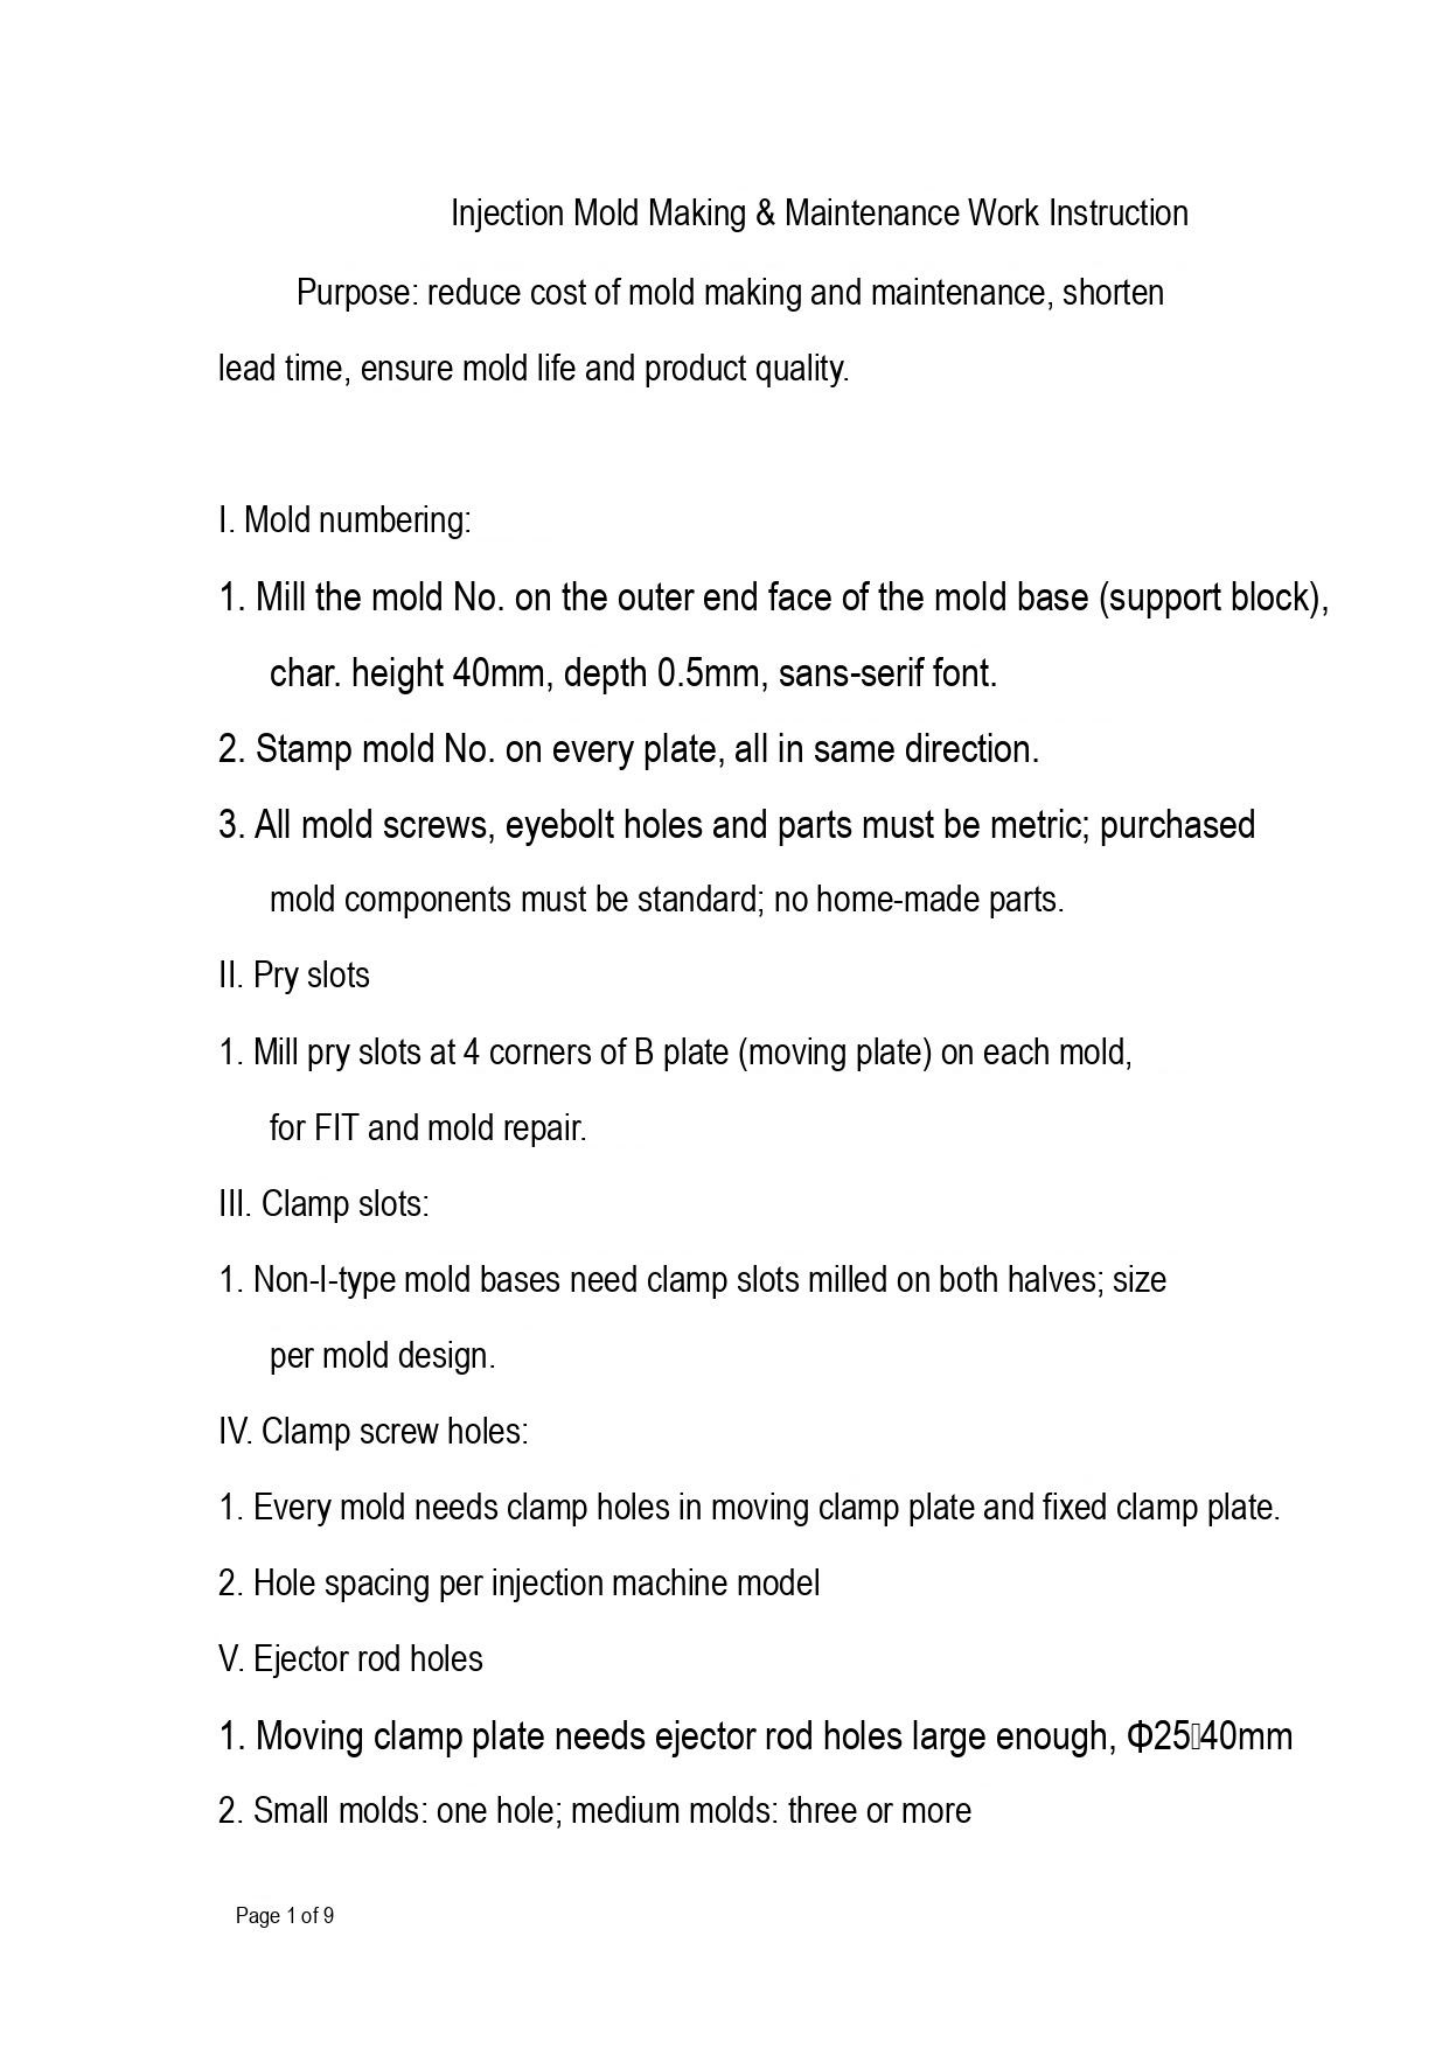Injection Mold Making & Maintenance Work Instruction

Purpose: reduce cost of mold making and maintenance, shorten lead time, ensure mold life and product quality.

I. Mold numbering:

1. Mill the mold No. on the outer end face of the mold base (support block), char. height 40mm, depth 0.5mm, sans-serif font.

2. Stamp mold No. on every plate, all in same direction.

3. All mold screws, eyebolt holes and parts must be metric; purchased mold components must be standard; no home-made parts.

II. Pry slots

1. Mill pry slots at 4 corners of B plate (moving plate) on each mold, for FIT and mold repair.

III. Clamp slots:

1. Non-I-type mold bases need clamp slots milled on both halves; size per mold design.

IV. Clamp screw holes:

1. Every mold needs clamp holes in moving clamp plate and fixed clamp plate.

2. Hole spacing per injection machine model

V. Ejector rod holes

1. Moving clamp plate needs ejector rod holes large enough, Φ25 40mm

2. Small molds: one hole; medium molds: three or more

Page 1 of 9
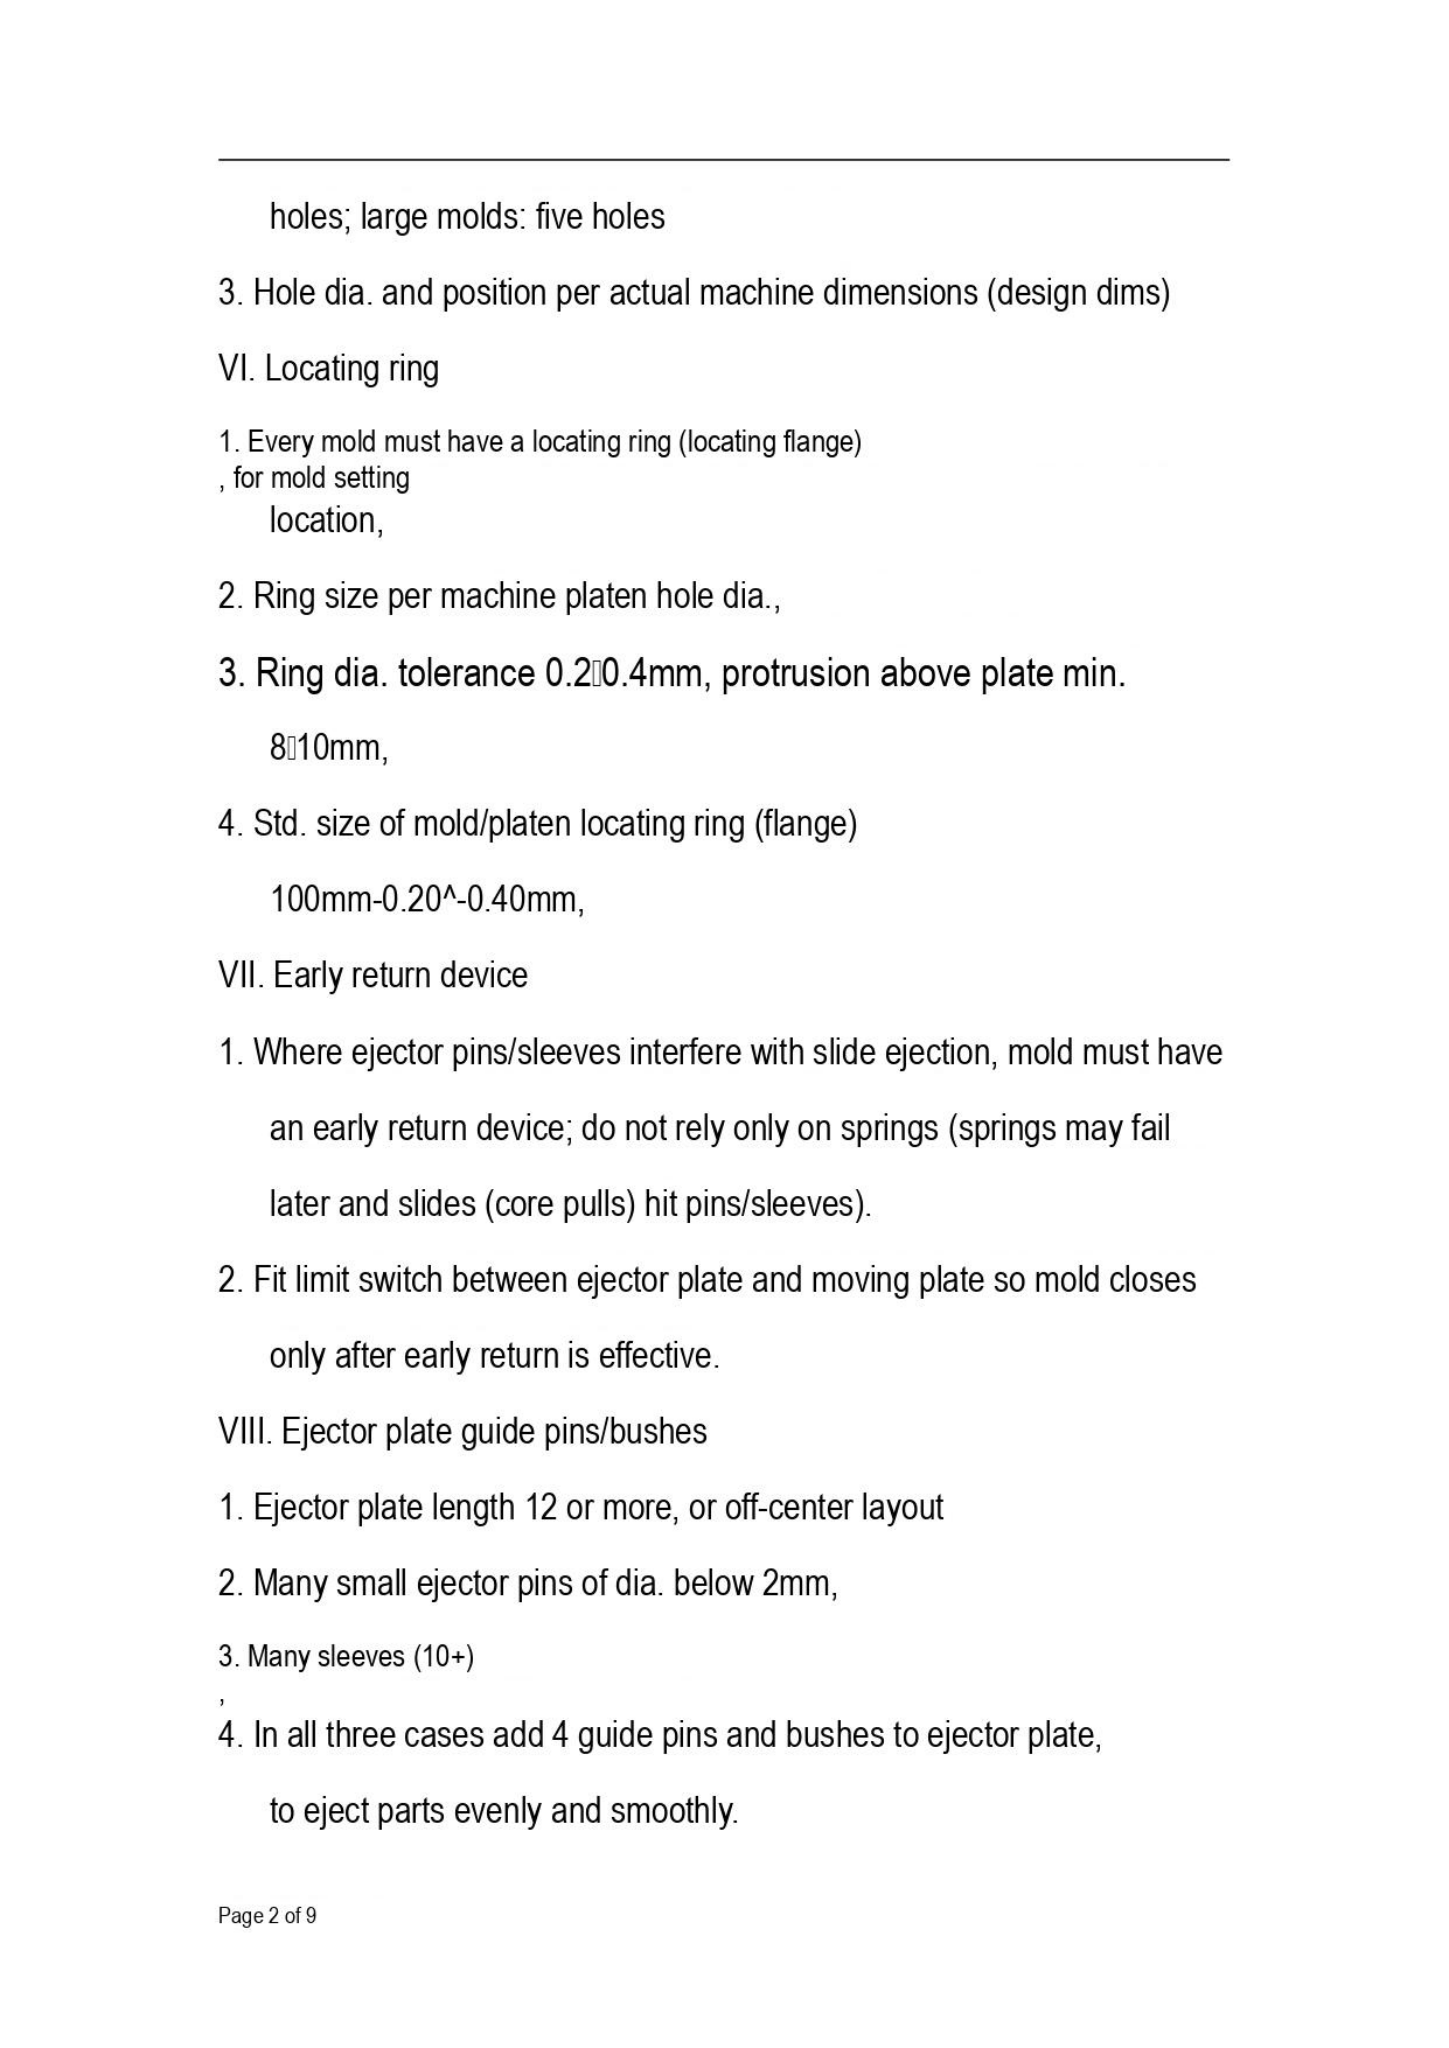holes; large molds: five holes

3. Hole dia. and position per actual machine dimensions (design dims)

VI. Locating ring

1. Every mold must have a locating ring (locating flange)
, for mold setting
location,

2. Ring size per machine platen hole dia.,

3. Ring dia. tolerance 0.2▯0.4mm, protrusion above plate min.
8▯10mm,

4. Std. size of mold/platen locating ring (flange)
100mm-0.20^-0.40mm,

VII. Early return device

1. Where ejector pins/sleeves interfere with slide ejection, mold must have an early return device; do not rely only on springs (springs may fail later and slides (core pulls) hit pins/sleeves).

2. Fit limit switch between ejector plate and moving plate so mold closes only after early return is effective.

VIII. Ejector plate guide pins/bushes

1. Ejector plate length 12 or more, or off-center layout

2. Many small ejector pins of dia. below 2mm,

3. Many sleeves (10+)
,

4. In all three cases add 4 guide pins and bushes to ejector plate, to eject parts evenly and smoothly.

Page 2 of 9
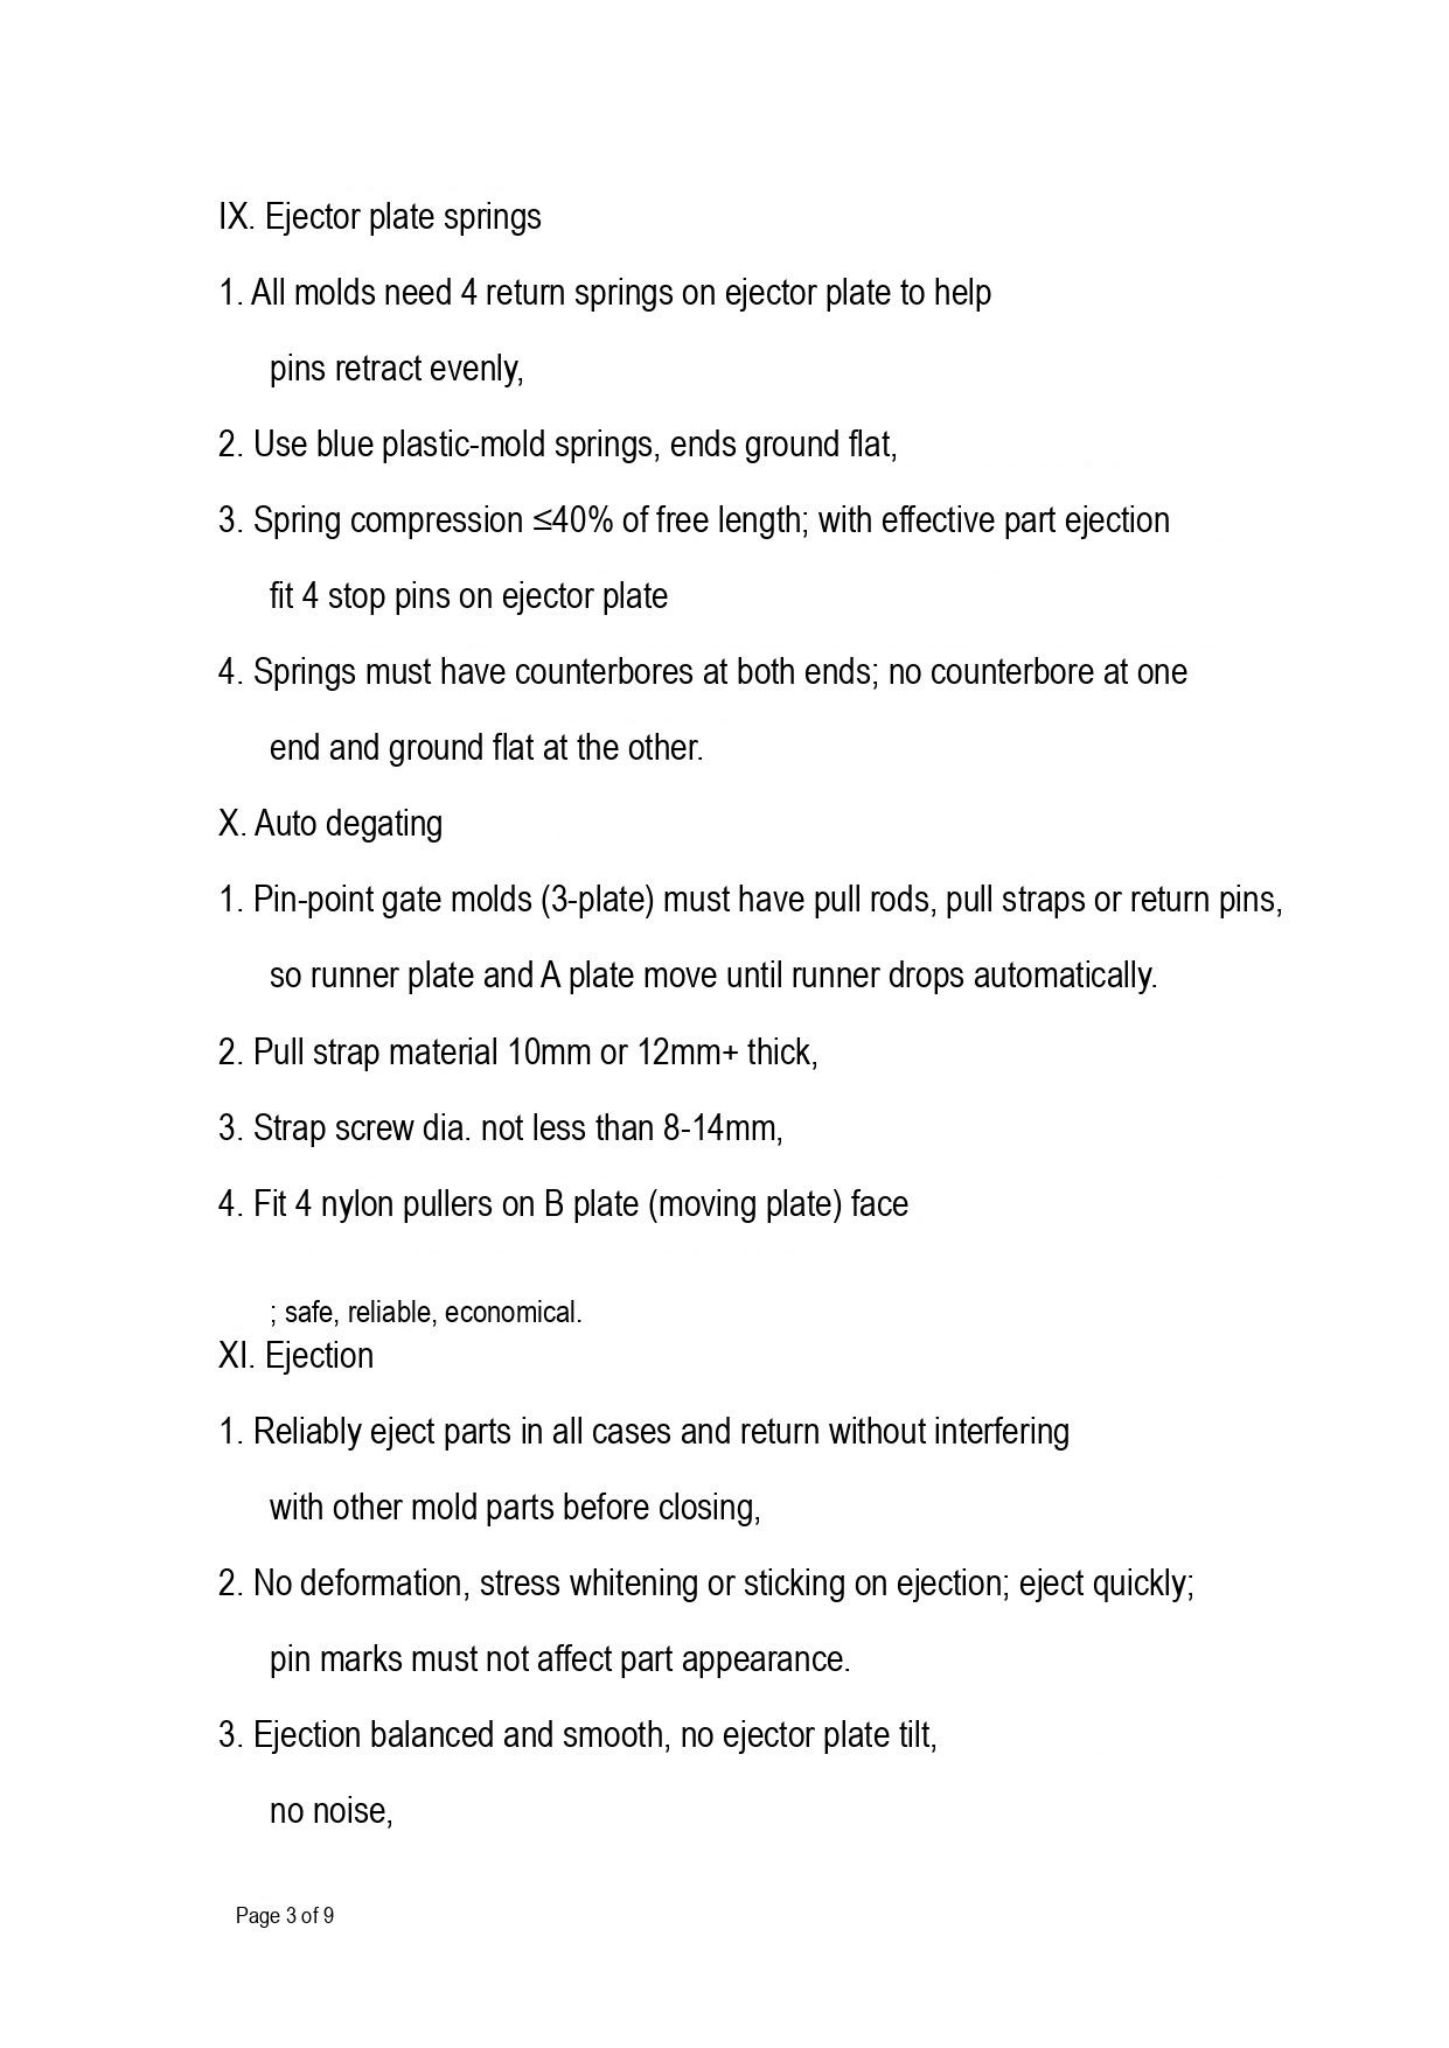IX. Ejector plate springs

1. All molds need 4 return springs on ejector plate to help
   pins retract evenly,

2. Use blue plastic-mold springs, ends ground flat,

3. Spring compression ≤40% of free length; with effective part ejection
   fit 4 stop pins on ejector plate

4. Springs must have counterbores at both ends; no counterbore at one
   end and ground flat at the other.

X. Auto degating

1. Pin-point gate molds (3-plate) must have pull rods, pull straps or return pins,
   so runner plate and A plate move until runner drops automatically.

2. Pull strap material 10mm or 12mm+ thick,

3. Strap screw dia. not less than 8-14mm,

4. Fit 4 nylon pullers on B plate (moving plate) face

   ; safe, reliable, economical.

XI. Ejection

1. Reliably eject parts in all cases and return without interfering
   with other mold parts before closing,

2. No deformation, stress whitening or sticking on ejection; eject quickly;
   pin marks must not affect part appearance.

3. Ejection balanced and smooth, no ejector plate tilt,
   no noise,

Page 3 of 9
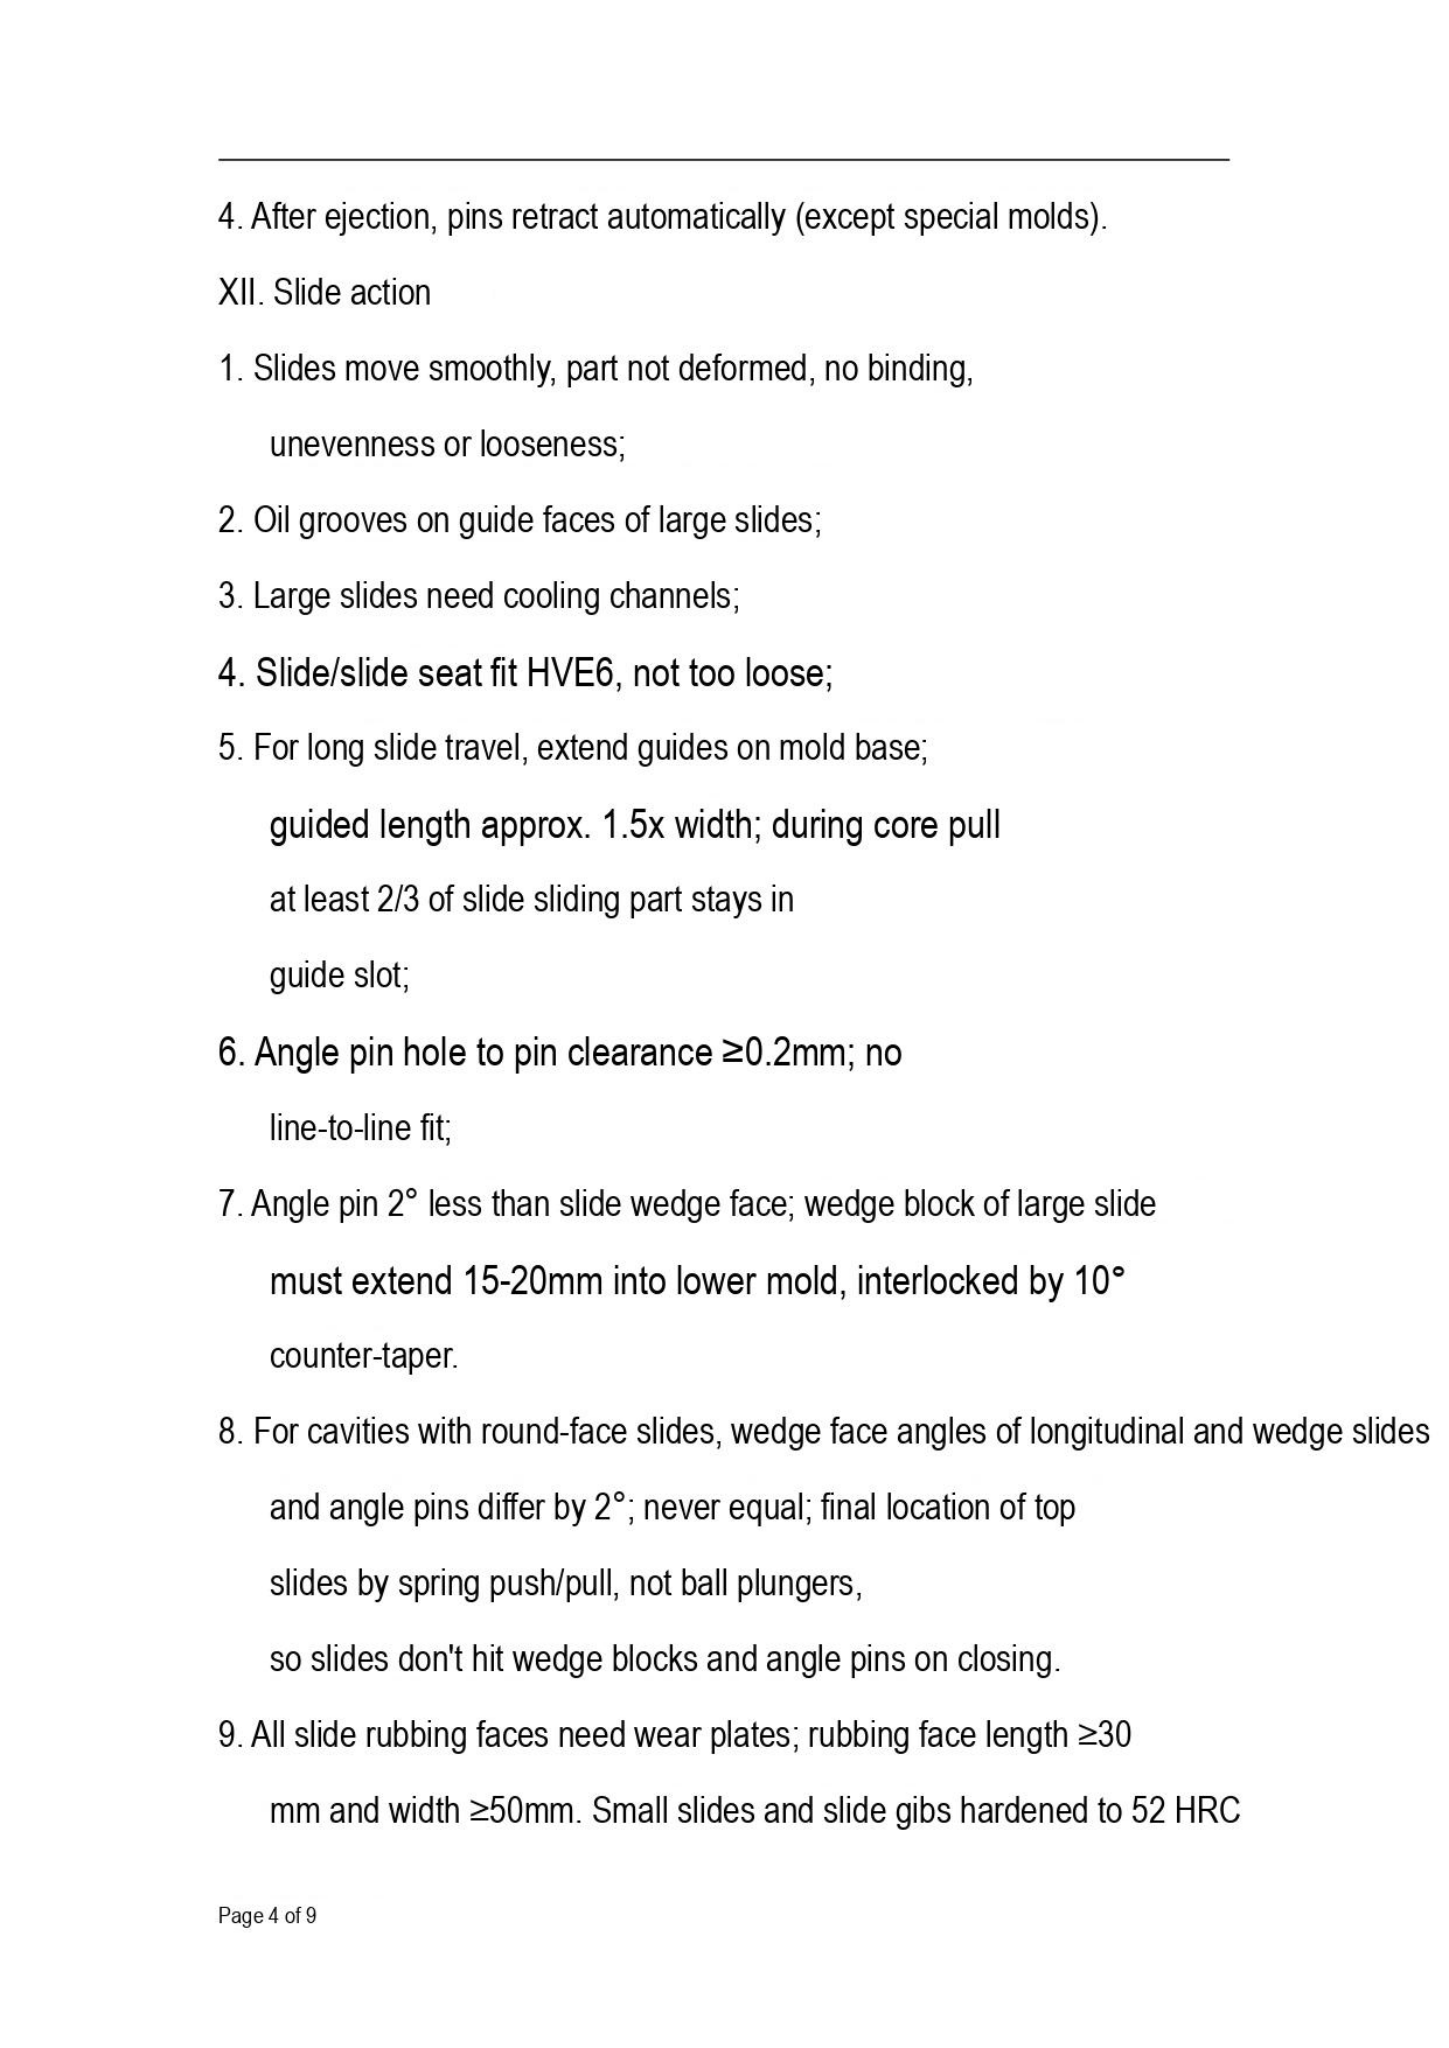4. After ejection, pins retract automatically (except special molds).

XII. Slide action

1. Slides move smoothly, part not deformed, no binding, unevenness or looseness;

2. Oil grooves on guide faces of large slides;

3. Large slides need cooling channels;

4. Slide/slide seat fit HVE6, not too loose;

5. For long slide travel, extend guides on mold base; guided length approx. 1.5x width; during core pull at least 2/3 of slide sliding part stays in guide slot;

6. Angle pin hole to pin clearance ≥0.2mm; no line-to-line fit;

7. Angle pin 2° less than slide wedge face; wedge block of large slide must extend 15-20mm into lower mold, interlocked by 10° counter-taper.

8. For cavities with round-face slides, wedge face angles of longitudinal and wedge slides and angle pins differ by 2°; never equal; final location of top slides by spring push/pull, not ball plungers, so slides don't hit wedge blocks and angle pins on closing.

9. All slide rubbing faces need wear plates; rubbing face length ≥30 mm and width ≥50mm. Small slides and slide gibs hardened to 52 HRC

Page 4 of 9
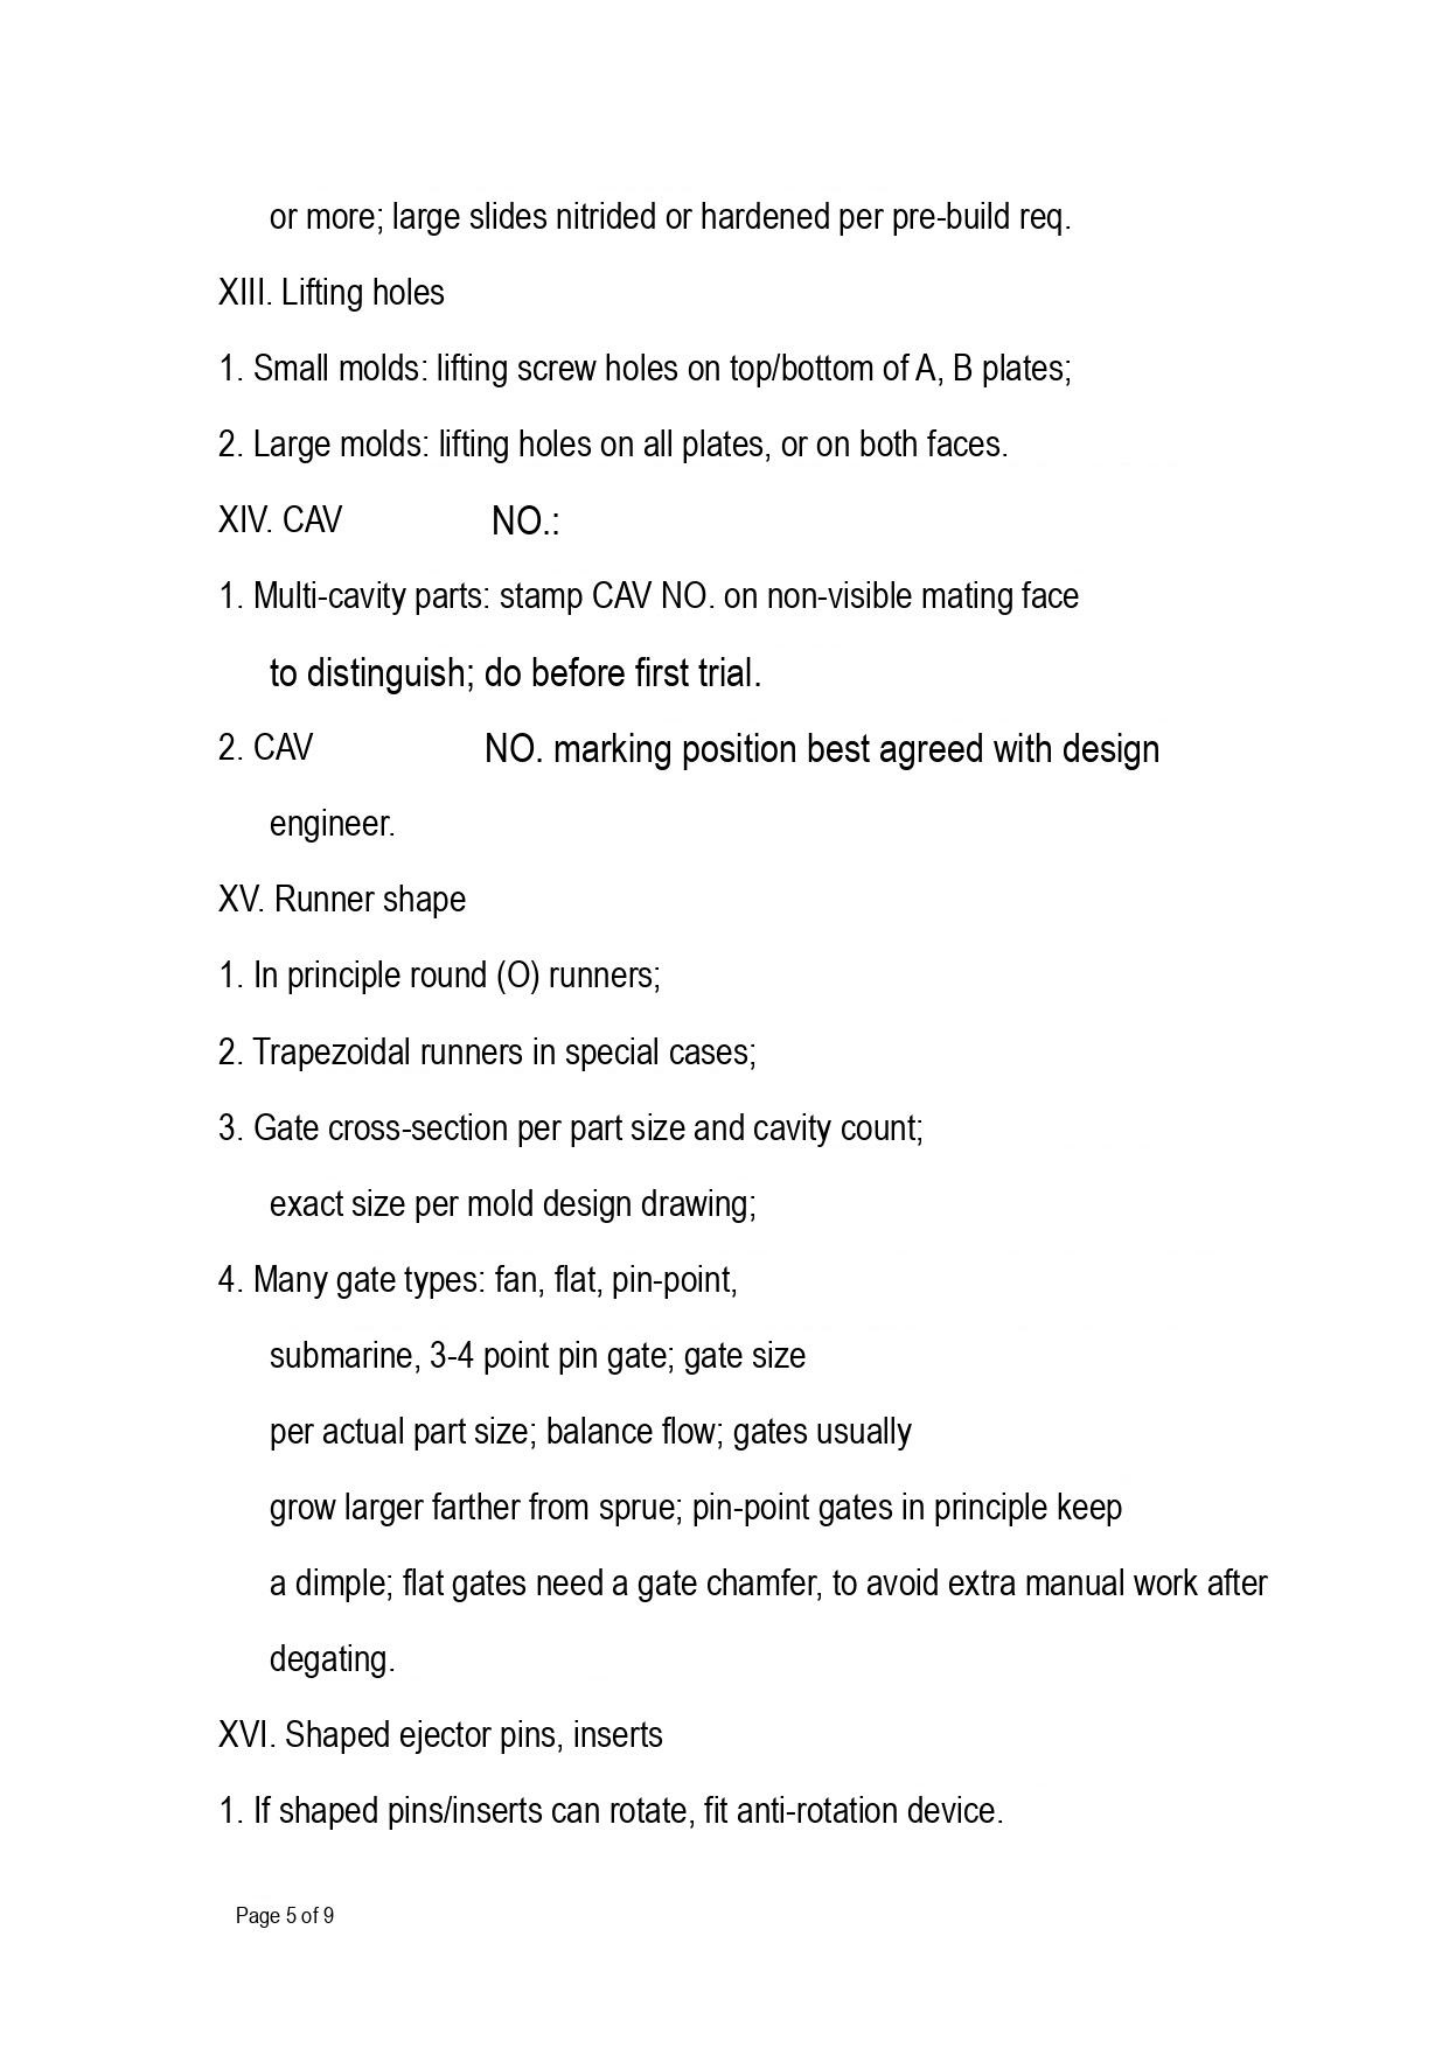or more; large slides nitrided or hardened per pre-build req.

XIII. Lifting holes

1. Small molds: lifting screw holes on top/bottom of A, B plates;

2. Large molds: lifting holes on all plates, or on both faces.

XIV. CAV NO.:

1. Multi-cavity parts: stamp CAV NO. on non-visible mating face to distinguish; do before first trial.

2. CAV NO. marking position best agreed with design engineer.

XV. Runner shape

1. In principle round (O) runners;

2. Trapezoidal runners in special cases;

3. Gate cross-section per part size and cavity count; exact size per mold design drawing;

4. Many gate types: fan, flat, pin-point, submarine, 3-4 point pin gate; gate size per actual part size; balance flow; gates usually grow larger farther from sprue; pin-point gates in principle keep a dimple; flat gates need a gate chamfer, to avoid extra manual work after degating.

XVI. Shaped ejector pins, inserts

1. If shaped pins/inserts can rotate, fit anti-rotation device.

Page 5 of 9
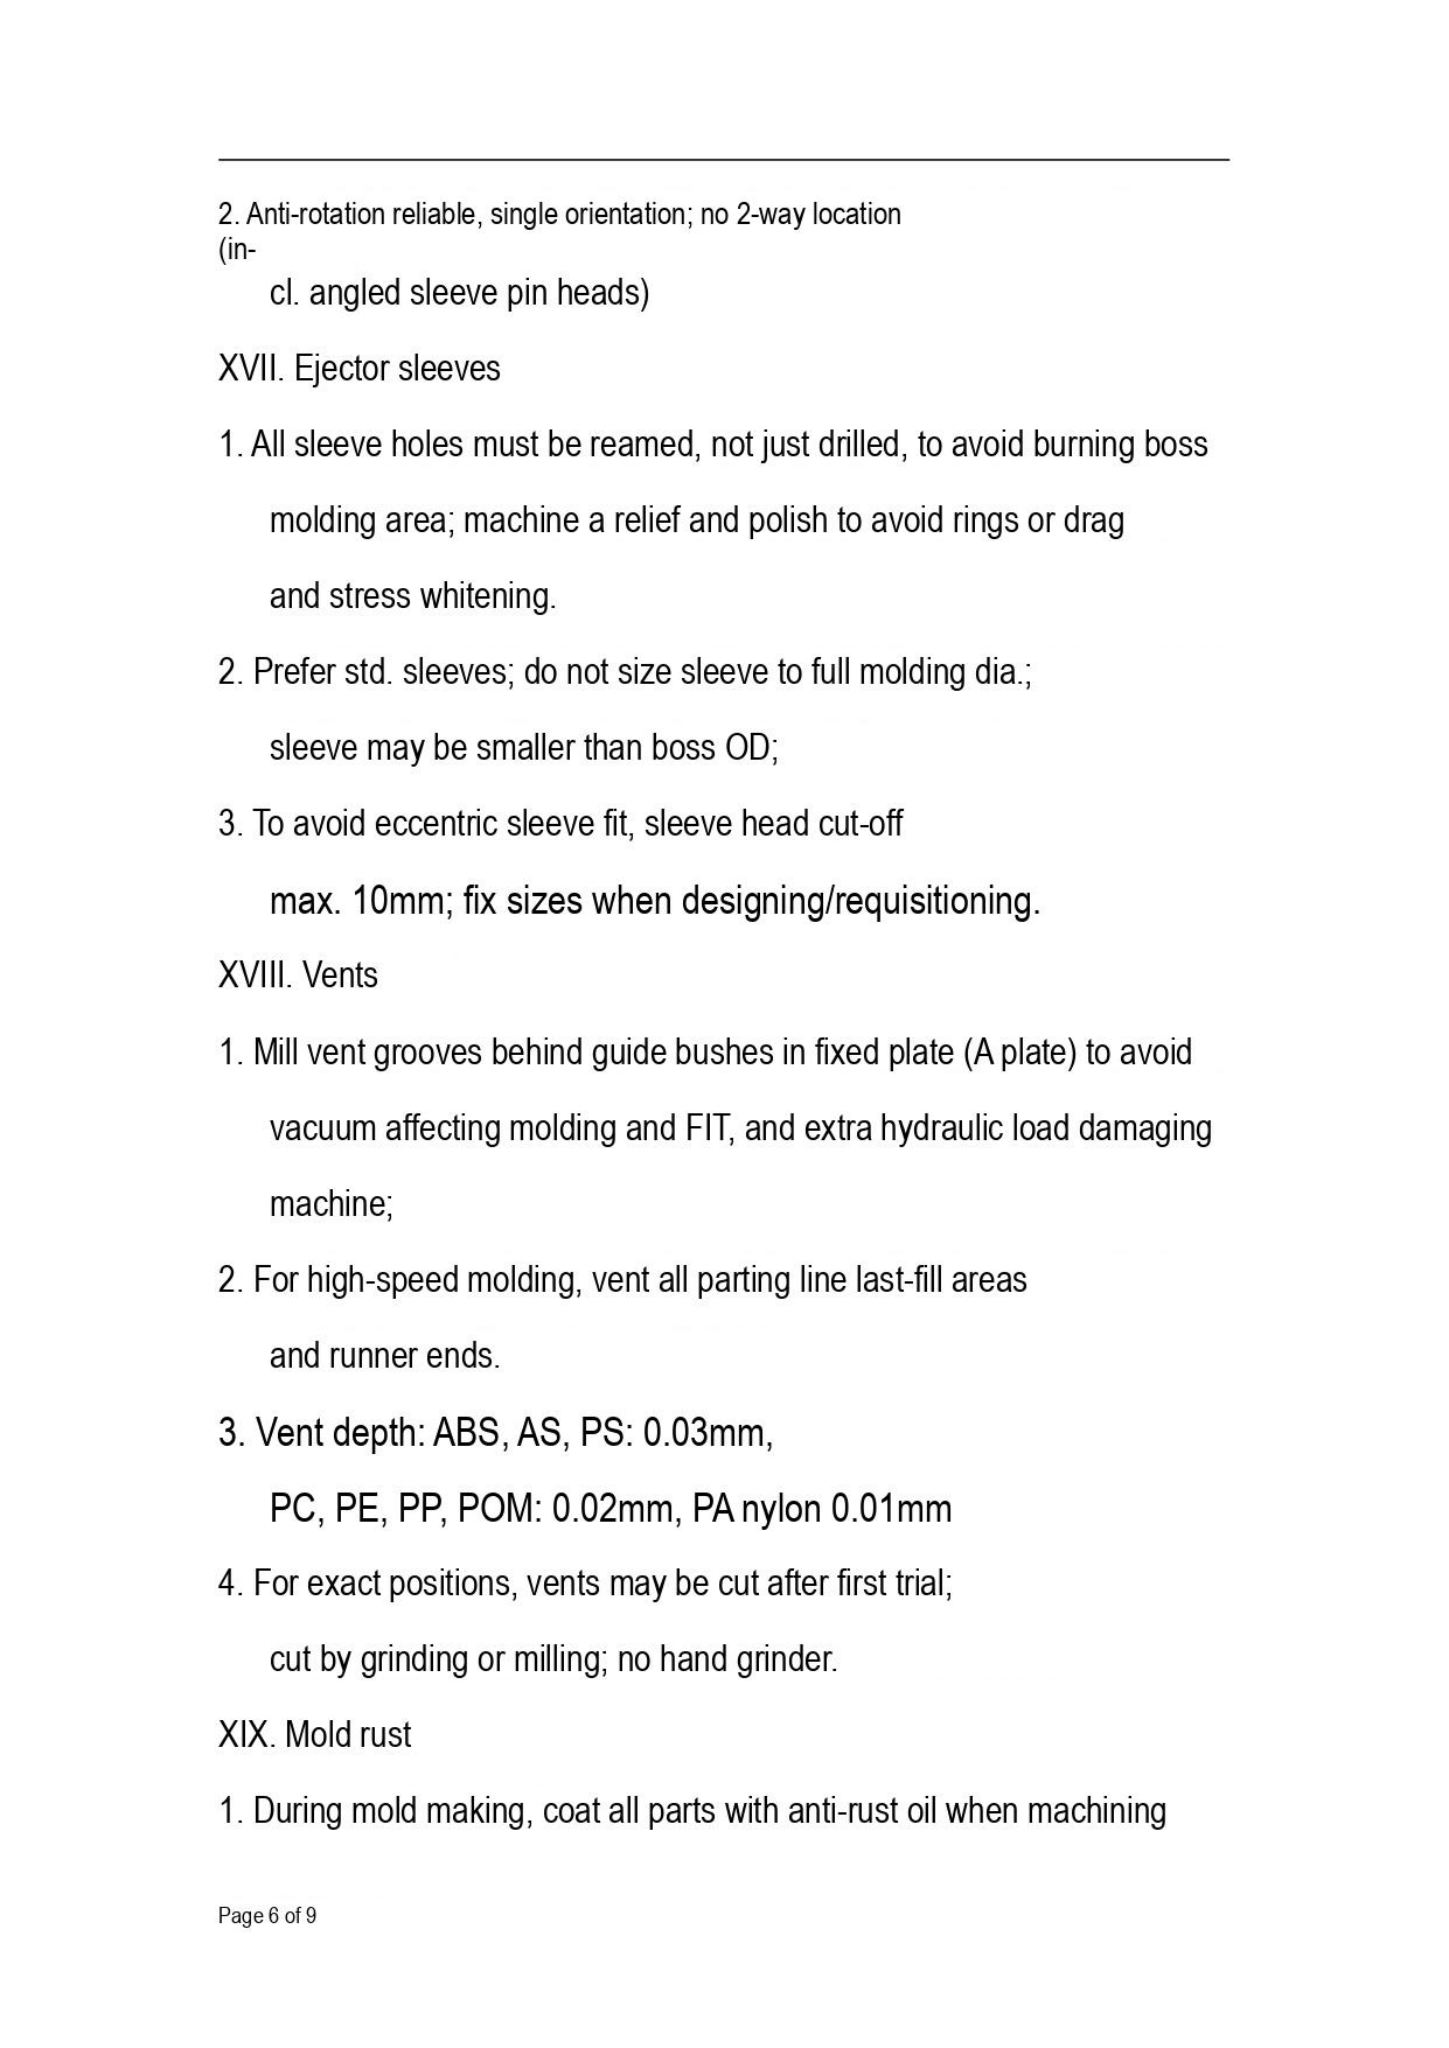2. Anti-rotation reliable, single orientation; no 2-way location (in-
cl. angled sleeve pin heads)

XVII. Ejector sleeves

1. All sleeve holes must be reamed, not just drilled, to avoid burning boss molding area; machine a relief and polish to avoid rings or drag and stress whitening.

2. Prefer std. sleeves; do not size sleeve to full molding dia.; sleeve may be smaller than boss OD;

3. To avoid eccentric sleeve fit, sleeve head cut-off max. 10mm; fix sizes when designing/requisitioning.

XVIII. Vents

1. Mill vent grooves behind guide bushes in fixed plate (A plate) to avoid vacuum affecting molding and FIT, and extra hydraulic load damaging machine;

2. For high-speed molding, vent all parting line last-fill areas and runner ends.

3. Vent depth: ABS, AS, PS: 0.03mm, PC, PE, PP, POM: 0.02mm, PA nylon 0.01mm

4. For exact positions, vents may be cut after first trial; cut by grinding or milling; no hand grinder.

XIX. Mold rust

1. During mold making, coat all parts with anti-rust oil when machining

Page 6 of 9
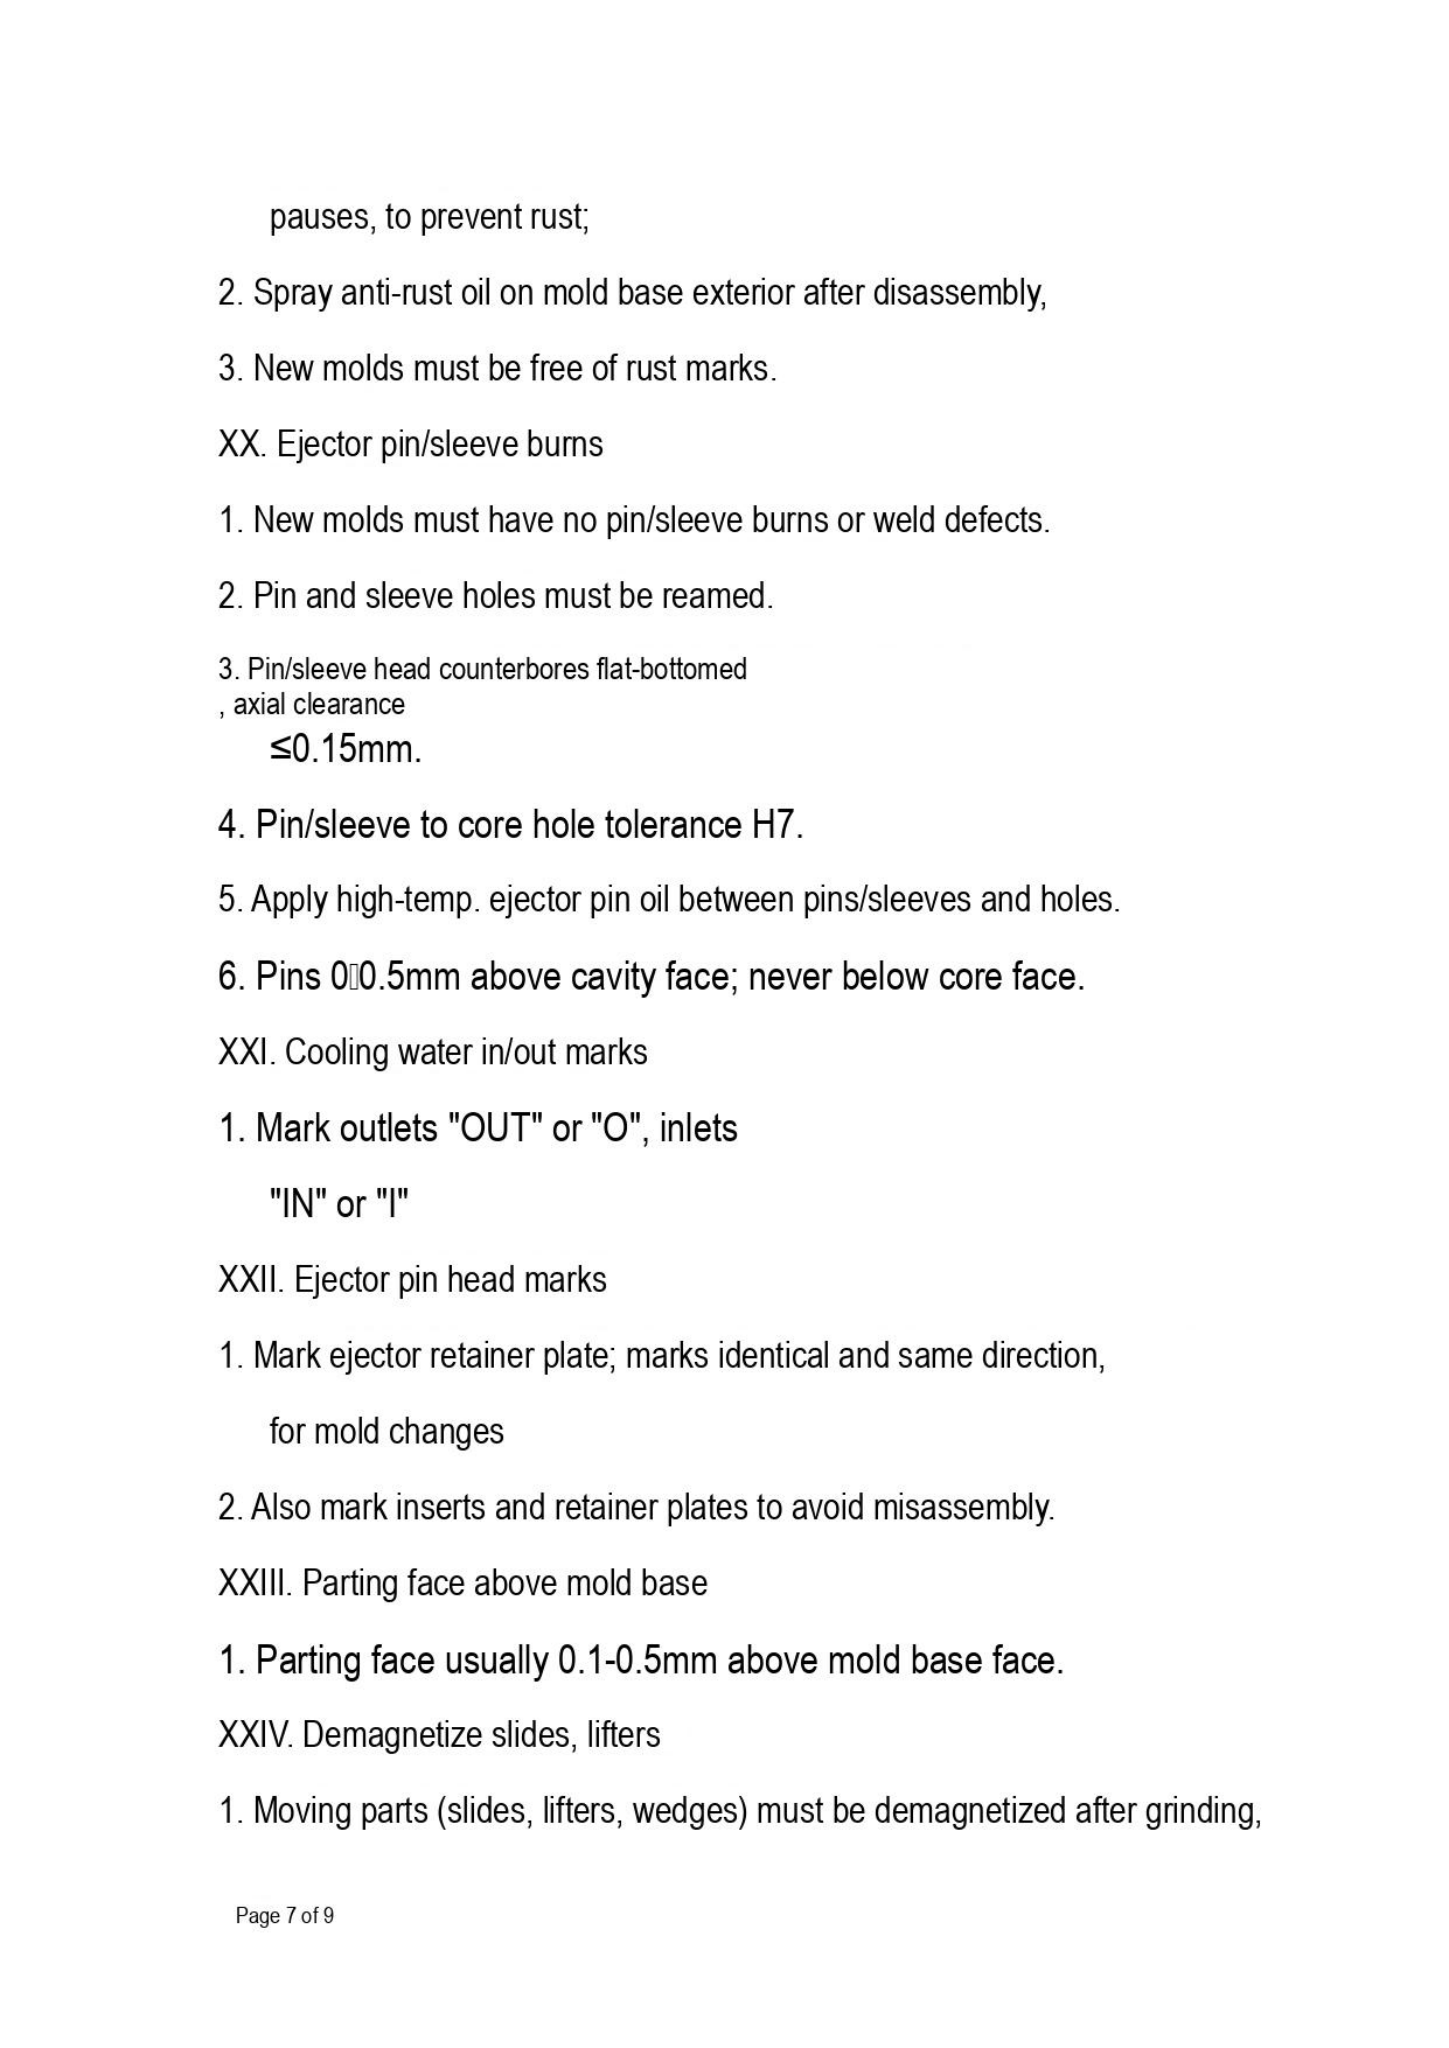pauses, to prevent rust;

2. Spray anti-rust oil on mold base exterior after disassembly,

3. New molds must be free of rust marks.

XX. Ejector pin/sleeve burns

1. New molds must have no pin/sleeve burns or weld defects.

2. Pin and sleeve holes must be reamed.

3. Pin/sleeve head counterbores flat-bottomed
, axial clearance
≤0.15mm.

4. Pin/sleeve to core hole tolerance H7.

5. Apply high-temp. ejector pin oil between pins/sleeves and holes.

6. Pins 0 0.5mm above cavity face; never below core face.

XXI. Cooling water in/out marks

1. Mark outlets "OUT" or "O", inlets
"IN" or "I"

XXII. Ejector pin head marks

1. Mark ejector retainer plate; marks identical and same direction,
for mold changes

2. Also mark inserts and retainer plates to avoid misassembly.

XXIII. Parting face above mold base

1. Parting face usually 0.1-0.5mm above mold base face.

XXIV. Demagnetize slides, lifters

1. Moving parts (slides, lifters, wedges) must be demagnetized after grinding,

Page 7 of 9